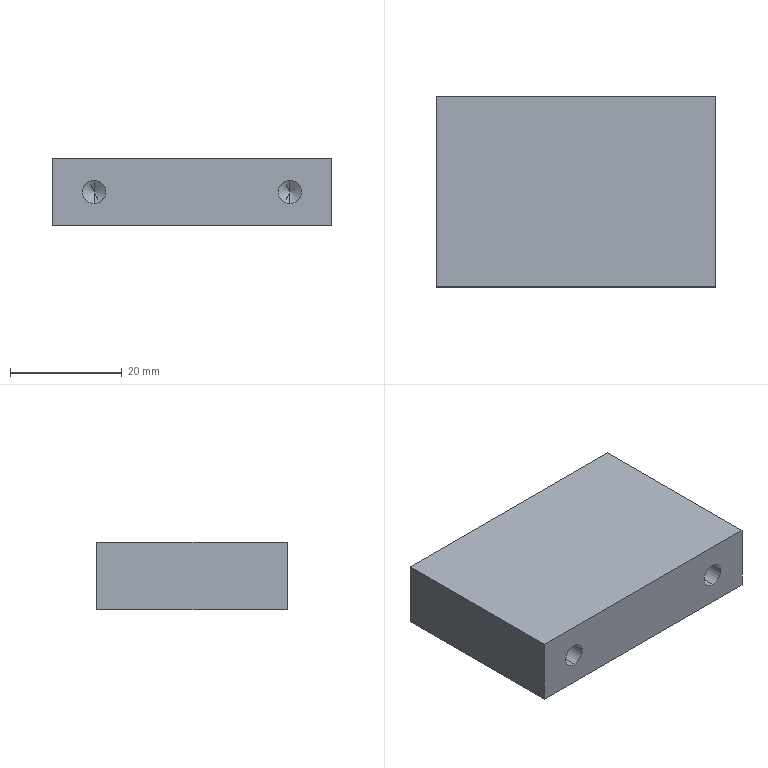Part | SolidWorks | features Extrusion 1, HoleWzd 1, MirrorPattern 1 | 1 solid | 22 faces | box 50 x 34 x 12 mm | volume 19690 mm3 | cylinder 8 | cone 8 | plane 6 | commonest cylinder face diameters 4.2 x8
STEP:
#1=CARTESIAN_POINT('',(-17.5,4.6,-2.1));
#2=VERTEX_POINT('',#1);
#3=CARTESIAN_POINT('',(-17.5,4.6,2.1));
#4=VERTEX_POINT('',#3);
#5=CARTESIAN_POINT('',(-17.5,4.6,0.));
#6=DIRECTION('',(0.,1.,0.));
#7=DIRECTION('',(0.,0.,1.));
#8=AXIS2_PLACEMENT_3D('',#5,#6,#7);
#9=CIRCLE('',#8,2.1);
#10=EDGE_CURVE('',#2,#4,#9,.T.);
#11=ORIENTED_EDGE('',*,*,#10,.F.);
#12=CARTESIAN_POINT('',(-17.5,17.,-2.1));
#13=VERTEX_POINT('',#12);
#14=CARTESIAN_POINT('',(-17.5,17.,-2.1));
#15=DIRECTION('',(0.,1.,0.));
#16=VECTOR('',#15,1000.);
#17=LINE('',#14,#16);
#18=EDGE_CURVE('',#2,#13,#17,.T.);
#19=ORIENTED_EDGE('',*,*,#18,.T.);
#20=CARTESIAN_POINT('',(-17.5,17.,2.1));
#21=VERTEX_POINT('',#20);
#22=CARTESIAN_POINT('',(-17.5,17.,0.));
#23=DIRECTION('',(0.,1.,0.));
#24=DIRECTION('',(0.,0.,1.));
#25=AXIS2_PLACEMENT_3D('',#22,#23,#24);
#26=CIRCLE('',#25,2.1);
#27=EDGE_CURVE('',#13,#21,#26,.T.);
#28=ORIENTED_EDGE('',*,*,#27,.T.);
#29=CARTESIAN_POINT('',(-17.5,17.,2.1));
#30=DIRECTION('',(0.,1.,0.));
#31=VECTOR('',#30,1000.);
#32=LINE('',#29,#31);
#33=EDGE_CURVE('',#4,#21,#32,.T.);
#34=ORIENTED_EDGE('',*,*,#33,.F.);
#35=EDGE_LOOP('',(#11,#19,#28,#34));
#36=FACE_OUTER_BOUND('',#35,.T.);
#37=CARTESIAN_POINT('',(-17.5,17.,0.));
#38=DIRECTION('',(0.,1.,0.));
#39=DIRECTION('',(0.,0.,1.));
#40=AXIS2_PLACEMENT_3D('',#37,#38,#39);
#41=CYLINDRICAL_SURFACE('',#40,2.1);
#42=ADVANCED_FACE('',(#36),#41,.F.);
#43=CARTESIAN_POINT('',(-17.5,3.338,0.));
#44=VERTEX_POINT('',#43);
#45=CARTESIAN_POINT('',(-17.5,4.6,2.1));
#46=DIRECTION('',(0.,0.515,0.8572));
#47=VECTOR('',#46,1000.);
#48=LINE('',#45,#47);
#49=EDGE_CURVE('',#44,#4,#48,.T.);
#50=ORIENTED_EDGE('',*,*,#49,.F.);
#51=CARTESIAN_POINT('',(-17.5,4.6,-2.1));
#52=DIRECTION('',(0.,0.515,-0.8572));
#53=VECTOR('',#52,1000.);
#54=LINE('',#51,#53);
#55=EDGE_CURVE('',#44,#2,#54,.T.);
#56=ORIENTED_EDGE('',*,*,#55,.T.);
#57=ORIENTED_EDGE('',*,*,#10,.T.);
#58=EDGE_LOOP('',(#50,#56,#57));
#59=FACE_OUTER_BOUND('',#58,.T.);
#60=CARTESIAN_POINT('',(-17.5,4.6,0.));
#61=DIRECTION('',(0.,1.,0.));
#62=DIRECTION('',(0.,0.,1.));
#63=AXIS2_PLACEMENT_3D('',#60,#61,#62);
#64=CONICAL_SURFACE('',#63,2.1,1.03);
#65=ADVANCED_FACE('',(#59),#64,.F.);
#66=CARTESIAN_POINT('',(17.5,4.6,-2.1));
#67=VERTEX_POINT('',#66);
#68=CARTESIAN_POINT('',(17.5,4.6,2.1));
#69=VERTEX_POINT('',#68);
#70=CARTESIAN_POINT('',(17.5,4.6,0.));
#71=DIRECTION('',(0.,1.,0.));
#72=DIRECTION('',(0.,0.,1.));
#73=AXIS2_PLACEMENT_3D('',#70,#71,#72);
#74=CIRCLE('',#73,2.1);
#75=EDGE_CURVE('',#67,#69,#74,.T.);
#76=ORIENTED_EDGE('',*,*,#75,.F.);
#77=CARTESIAN_POINT('',(17.5,17.,-2.1));
#78=VERTEX_POINT('',#77);
#79=CARTESIAN_POINT('',(17.5,17.,-2.1));
#80=DIRECTION('',(0.,1.,0.));
#81=VECTOR('',#80,1000.);
#82=LINE('',#79,#81);
#83=EDGE_CURVE('',#67,#78,#82,.T.);
#84=ORIENTED_EDGE('',*,*,#83,.T.);
#85=CARTESIAN_POINT('',(17.5,17.,2.1));
#86=VERTEX_POINT('',#85);
#87=CARTESIAN_POINT('',(17.5,17.,0.));
#88=DIRECTION('',(0.,1.,0.));
#89=DIRECTION('',(0.,0.,1.));
#90=AXIS2_PLACEMENT_3D('',#87,#88,#89);
#91=CIRCLE('',#90,2.1);
#92=EDGE_CURVE('',#78,#86,#91,.T.);
#93=ORIENTED_EDGE('',*,*,#92,.T.);
#94=CARTESIAN_POINT('',(17.5,17.,2.1));
#95=DIRECTION('',(0.,1.,0.));
#96=VECTOR('',#95,1000.);
#97=LINE('',#94,#96);
#98=EDGE_CURVE('',#69,#86,#97,.T.);
#99=ORIENTED_EDGE('',*,*,#98,.F.);
#100=EDGE_LOOP('',(#76,#84,#93,#99));
#101=FACE_OUTER_BOUND('',#100,.T.);
#102=CARTESIAN_POINT('',(17.5,17.,0.));
#103=DIRECTION('',(0.,1.,0.));
#104=DIRECTION('',(0.,0.,1.));
#105=AXIS2_PLACEMENT_3D('',#102,#103,#104);
#106=CYLINDRICAL_SURFACE('',#105,2.1);
#107=ADVANCED_FACE('',(#101),#106,.F.);
#108=CARTESIAN_POINT('',(17.5,3.338,0.));
#109=VERTEX_POINT('',#108);
#110=CARTESIAN_POINT('',(17.5,4.6,2.1));
#111=DIRECTION('',(0.,0.515,0.8572));
#112=VECTOR('',#111,1000.);
#113=LINE('',#110,#112);
#114=EDGE_CURVE('',#109,#69,#113,.T.);
#115=ORIENTED_EDGE('',*,*,#114,.F.);
#116=CARTESIAN_POINT('',(17.5,4.6,-2.1));
#117=DIRECTION('',(0.,0.515,-0.8572));
#118=VECTOR('',#117,1000.);
#119=LINE('',#116,#118);
#120=EDGE_CURVE('',#109,#67,#119,.T.);
#121=ORIENTED_EDGE('',*,*,#120,.T.);
#122=ORIENTED_EDGE('',*,*,#75,.T.);
#123=EDGE_LOOP('',(#115,#121,#122));
#124=FACE_OUTER_BOUND('',#123,.T.);
#125=CARTESIAN_POINT('',(17.5,4.6,0.));
#126=DIRECTION('',(0.,1.,0.));
#127=DIRECTION('',(0.,0.,1.));
#128=AXIS2_PLACEMENT_3D('',#125,#126,#127);
#129=CONICAL_SURFACE('',#128,2.1,1.03);
#130=ADVANCED_FACE('',(#124),#129,.F.);
#131=CARTESIAN_POINT('',(-17.5,-4.6,2.1));
#132=VERTEX_POINT('',#131);
#133=CARTESIAN_POINT('',(-17.5,-4.6,-2.1));
#134=VERTEX_POINT('',#133);
#135=CARTESIAN_POINT('',(-17.5,-4.6,0.));
#136=DIRECTION('',(0.,-1.,0.));
#137=DIRECTION('',(0.,0.,-1.));
#138=AXIS2_PLACEMENT_3D('',#135,#136,#137);
#139=CIRCLE('',#138,2.1);
#140=EDGE_CURVE('',#132,#134,#139,.T.);
#141=ORIENTED_EDGE('',*,*,#140,.F.);
#142=CARTESIAN_POINT('',(-17.5,-17.,2.1));
#143=VERTEX_POINT('',#142);
#144=CARTESIAN_POINT('',(-17.5,-17.,2.1));
#145=DIRECTION('',(0.,-1.,0.));
#146=VECTOR('',#145,1000.);
#147=LINE('',#144,#146);
#148=EDGE_CURVE('',#132,#143,#147,.T.);
#149=ORIENTED_EDGE('',*,*,#148,.T.);
#150=CARTESIAN_POINT('',(-17.5,-17.,-2.1));
#151=VERTEX_POINT('',#150);
#152=CARTESIAN_POINT('',(-17.5,-17.,0.));
#153=DIRECTION('',(0.,-1.,0.));
#154=DIRECTION('',(0.,0.,-1.));
#155=AXIS2_PLACEMENT_3D('',#152,#153,#154);
#156=CIRCLE('',#155,2.1);
#157=EDGE_CURVE('',#143,#151,#156,.T.);
#158=ORIENTED_EDGE('',*,*,#157,.T.);
#159=CARTESIAN_POINT('',(-17.5,-17.,-2.1));
#160=DIRECTION('',(0.,-1.,0.));
#161=VECTOR('',#160,1000.);
#162=LINE('',#159,#161);
#163=EDGE_CURVE('',#134,#151,#162,.T.);
#164=ORIENTED_EDGE('',*,*,#163,.F.);
#165=EDGE_LOOP('',(#141,#149,#158,#164));
#166=FACE_OUTER_BOUND('',#165,.T.);
#167=CARTESIAN_POINT('',(-17.5,-17.,0.));
#168=DIRECTION('',(0.,-1.,0.));
#169=DIRECTION('',(0.,0.,-1.));
#170=AXIS2_PLACEMENT_3D('',#167,#168,#169);
#171=CYLINDRICAL_SURFACE('',#170,2.1);
#172=ADVANCED_FACE('',(#166),#171,.F.);
#173=CARTESIAN_POINT('',(-17.5,-3.338,0.));
#174=VERTEX_POINT('',#173);
#175=CARTESIAN_POINT('',(-17.5,-4.6,-2.1));
#176=DIRECTION('',(0.,-0.515,-0.8572));
#177=VECTOR('',#176,1000.);
#178=LINE('',#175,#177);
#179=EDGE_CURVE('',#174,#134,#178,.T.);
#180=ORIENTED_EDGE('',*,*,#179,.F.);
#181=CARTESIAN_POINT('',(-17.5,-4.6,2.1));
#182=DIRECTION('',(0.,-0.515,0.8572));
#183=VECTOR('',#182,1000.);
#184=LINE('',#181,#183);
#185=EDGE_CURVE('',#174,#132,#184,.T.);
#186=ORIENTED_EDGE('',*,*,#185,.T.);
#187=ORIENTED_EDGE('',*,*,#140,.T.);
#188=EDGE_LOOP('',(#180,#186,#187));
#189=FACE_OUTER_BOUND('',#188,.T.);
#190=CARTESIAN_POINT('',(-17.5,-4.6,0.));
#191=DIRECTION('',(0.,-1.,0.));
#192=DIRECTION('',(0.,0.,-1.));
#193=AXIS2_PLACEMENT_3D('',#190,#191,#192);
#194=CONICAL_SURFACE('',#193,2.1,1.03);
#195=ADVANCED_FACE('',(#189),#194,.F.);
#196=CARTESIAN_POINT('',(17.5,-4.6,2.1));
#197=VERTEX_POINT('',#196);
#198=CARTESIAN_POINT('',(17.5,-4.6,-2.1));
#199=VERTEX_POINT('',#198);
#200=CARTESIAN_POINT('',(17.5,-4.6,0.));
#201=DIRECTION('',(0.,-1.,0.));
#202=DIRECTION('',(0.,0.,-1.));
#203=AXIS2_PLACEMENT_3D('',#200,#201,#202);
#204=CIRCLE('',#203,2.1);
#205=EDGE_CURVE('',#197,#199,#204,.T.);
#206=ORIENTED_EDGE('',*,*,#205,.F.);
#207=CARTESIAN_POINT('',(17.5,-17.,2.1));
#208=VERTEX_POINT('',#207);
#209=CARTESIAN_POINT('',(17.5,-17.,2.1));
#210=DIRECTION('',(0.,-1.,0.));
#211=VECTOR('',#210,1000.);
#212=LINE('',#209,#211);
#213=EDGE_CURVE('',#197,#208,#212,.T.);
#214=ORIENTED_EDGE('',*,*,#213,.T.);
#215=CARTESIAN_POINT('',(17.5,-17.,-2.1));
#216=VERTEX_POINT('',#215);
#217=CARTESIAN_POINT('',(17.5,-17.,0.));
#218=DIRECTION('',(0.,-1.,0.));
#219=DIRECTION('',(0.,0.,-1.));
#220=AXIS2_PLACEMENT_3D('',#217,#218,#219);
#221=CIRCLE('',#220,2.1);
#222=EDGE_CURVE('',#208,#216,#221,.T.);
#223=ORIENTED_EDGE('',*,*,#222,.T.);
#224=CARTESIAN_POINT('',(17.5,-17.,-2.1));
#225=DIRECTION('',(0.,-1.,0.));
#226=VECTOR('',#225,1000.);
#227=LINE('',#224,#226);
#228=EDGE_CURVE('',#199,#216,#227,.T.);
#229=ORIENTED_EDGE('',*,*,#228,.F.);
#230=EDGE_LOOP('',(#206,#214,#223,#229));
#231=FACE_OUTER_BOUND('',#230,.T.);
#232=CARTESIAN_POINT('',(17.5,-17.,0.));
#233=DIRECTION('',(0.,-1.,0.));
#234=DIRECTION('',(0.,0.,-1.));
#235=AXIS2_PLACEMENT_3D('',#232,#233,#234);
#236=CYLINDRICAL_SURFACE('',#235,2.1);
#237=ADVANCED_FACE('',(#231),#236,.F.);
#238=CARTESIAN_POINT('',(17.5,-3.338,0.));
#239=VERTEX_POINT('',#238);
#240=CARTESIAN_POINT('',(17.5,-4.6,-2.1));
#241=DIRECTION('',(0.,-0.515,-0.8572));
#242=VECTOR('',#241,1000.);
#243=LINE('',#240,#242);
#244=EDGE_CURVE('',#239,#199,#243,.T.);
#245=ORIENTED_EDGE('',*,*,#244,.F.);
#246=CARTESIAN_POINT('',(17.5,-4.6,2.1));
#247=DIRECTION('',(0.,-0.515,0.8572));
#248=VECTOR('',#247,1000.);
#249=LINE('',#246,#248);
#250=EDGE_CURVE('',#239,#197,#249,.T.);
#251=ORIENTED_EDGE('',*,*,#250,.T.);
#252=ORIENTED_EDGE('',*,*,#205,.T.);
#253=EDGE_LOOP('',(#245,#251,#252));
#254=FACE_OUTER_BOUND('',#253,.T.);
#255=CARTESIAN_POINT('',(17.5,-4.6,0.));
#256=DIRECTION('',(0.,-1.,0.));
#257=DIRECTION('',(0.,0.,-1.));
#258=AXIS2_PLACEMENT_3D('',#255,#256,#257);
#259=CONICAL_SURFACE('',#258,2.1,1.03);
#260=ADVANCED_FACE('',(#254),#259,.F.);
#261=CARTESIAN_POINT('',(25.,-17.,-6.));
#262=VERTEX_POINT('',#261);
#263=CARTESIAN_POINT('',(25.,17.,-6.));
#264=VERTEX_POINT('',#263);
#265=CARTESIAN_POINT('',(25.,-17.,-6.));
#266=DIRECTION('',(0.,1.,0.));
#267=VECTOR('',#266,1000.);
#268=LINE('',#265,#267);
#269=EDGE_CURVE('',#262,#264,#268,.T.);
#270=ORIENTED_EDGE('',*,*,#269,.T.);
#271=CARTESIAN_POINT('',(25.,17.,6.));
#272=VERTEX_POINT('',#271);
#273=CARTESIAN_POINT('',(25.,17.,6.));
#274=DIRECTION('',(0.,0.,-1.));
#275=VECTOR('',#274,1000.);
#276=LINE('',#273,#275);
#277=EDGE_CURVE('',#272,#264,#276,.T.);
#278=ORIENTED_EDGE('',*,*,#277,.F.);
#279=CARTESIAN_POINT('',(25.,-17.,6.));
#280=VERTEX_POINT('',#279);
#281=CARTESIAN_POINT('',(25.,-17.,6.));
#282=DIRECTION('',(0.,1.,0.));
#283=VECTOR('',#282,1000.);
#284=LINE('',#281,#283);
#285=EDGE_CURVE('',#280,#272,#284,.T.);
#286=ORIENTED_EDGE('',*,*,#285,.F.);
#287=CARTESIAN_POINT('',(25.,-17.,6.));
#288=DIRECTION('',(0.,0.,-1.));
#289=VECTOR('',#288,1000.);
#290=LINE('',#287,#289);
#291=EDGE_CURVE('',#280,#262,#290,.T.);
#292=ORIENTED_EDGE('',*,*,#291,.T.);
#293=EDGE_LOOP('',(#270,#278,#286,#292));
#294=FACE_OUTER_BOUND('',#293,.T.);
#295=CARTESIAN_POINT('',(25.,-17.,6.));
#296=DIRECTION('',(-1.,0.,0.));
#297=DIRECTION('',(0.,0.,1.));
#298=AXIS2_PLACEMENT_3D('',#295,#296,#297);
#299=PLANE('',#298);
#300=ADVANCED_FACE('',(#294),#299,.F.);
#301=CARTESIAN_POINT('',(-17.5,17.,0.));
#302=DIRECTION('',(0.,1.,0.));
#303=DIRECTION('',(0.,0.,1.));
#304=AXIS2_PLACEMENT_3D('',#301,#302,#303);
#305=CIRCLE('',#304,2.1);
#306=EDGE_CURVE('',#21,#13,#305,.T.);
#307=ORIENTED_EDGE('',*,*,#306,.F.);
#308=ORIENTED_EDGE('',*,*,#27,.F.);
#309=EDGE_LOOP('',(#307,#308));
#310=FACE_BOUND('',#309,.T.);
#311=CARTESIAN_POINT('',(17.5,17.,0.));
#312=DIRECTION('',(0.,1.,0.));
#313=DIRECTION('',(0.,0.,1.));
#314=AXIS2_PLACEMENT_3D('',#311,#312,#313);
#315=CIRCLE('',#314,2.1);
#316=EDGE_CURVE('',#86,#78,#315,.T.);
#317=ORIENTED_EDGE('',*,*,#316,.F.);
#318=ORIENTED_EDGE('',*,*,#92,.F.);
#319=EDGE_LOOP('',(#317,#318));
#320=FACE_BOUND('',#319,.T.);
#321=CARTESIAN_POINT('',(-25.,17.,-6.));
#322=VERTEX_POINT('',#321);
#323=CARTESIAN_POINT('',(-25.,17.,-6.));
#324=DIRECTION('',(-1.,0.,0.));
#325=VECTOR('',#324,1000.);
#326=LINE('',#323,#325);
#327=EDGE_CURVE('',#264,#322,#326,.T.);
#328=ORIENTED_EDGE('',*,*,#327,.T.);
#329=CARTESIAN_POINT('',(-25.,17.,6.));
#330=VERTEX_POINT('',#329);
#331=CARTESIAN_POINT('',(-25.,17.,6.));
#332=DIRECTION('',(0.,0.,-1.));
#333=VECTOR('',#332,1000.);
#334=LINE('',#331,#333);
#335=EDGE_CURVE('',#330,#322,#334,.T.);
#336=ORIENTED_EDGE('',*,*,#335,.F.);
#337=CARTESIAN_POINT('',(-25.,17.,6.));
#338=DIRECTION('',(-1.,0.,0.));
#339=VECTOR('',#338,1000.);
#340=LINE('',#337,#339);
#341=EDGE_CURVE('',#272,#330,#340,.T.);
#342=ORIENTED_EDGE('',*,*,#341,.F.);
#343=ORIENTED_EDGE('',*,*,#277,.T.);
#344=EDGE_LOOP('',(#328,#336,#342,#343));
#345=FACE_OUTER_BOUND('',#344,.T.);
#346=CARTESIAN_POINT('',(-25.,17.,6.));
#347=DIRECTION('',(0.,-1.,0.));
#348=DIRECTION('',(0.,0.,-1.));
#349=AXIS2_PLACEMENT_3D('',#346,#347,#348);
#350=PLANE('',#349);
#351=ADVANCED_FACE('',(#310,#320,#345),#350,.F.);
#352=CARTESIAN_POINT('',(-25.,-17.,-6.));
#353=VERTEX_POINT('',#352);
#354=CARTESIAN_POINT('',(-25.,-17.,-6.));
#355=DIRECTION('',(0.,-1.,0.));
#356=VECTOR('',#355,1000.);
#357=LINE('',#354,#356);
#358=EDGE_CURVE('',#322,#353,#357,.T.);
#359=ORIENTED_EDGE('',*,*,#358,.T.);
#360=CARTESIAN_POINT('',(-25.,-17.,6.));
#361=VERTEX_POINT('',#360);
#362=CARTESIAN_POINT('',(-25.,-17.,6.));
#363=DIRECTION('',(0.,0.,-1.));
#364=VECTOR('',#363,1000.);
#365=LINE('',#362,#364);
#366=EDGE_CURVE('',#361,#353,#365,.T.);
#367=ORIENTED_EDGE('',*,*,#366,.F.);
#368=CARTESIAN_POINT('',(-25.,-17.,6.));
#369=DIRECTION('',(0.,-1.,0.));
#370=VECTOR('',#369,1000.);
#371=LINE('',#368,#370);
#372=EDGE_CURVE('',#330,#361,#371,.T.);
#373=ORIENTED_EDGE('',*,*,#372,.F.);
#374=ORIENTED_EDGE('',*,*,#335,.T.);
#375=EDGE_LOOP('',(#359,#367,#373,#374));
#376=FACE_OUTER_BOUND('',#375,.T.);
#377=CARTESIAN_POINT('',(-25.,-17.,6.));
#378=DIRECTION('',(1.,0.,0.));
#379=DIRECTION('',(0.,0.,-1.));
#380=AXIS2_PLACEMENT_3D('',#377,#378,#379);
#381=PLANE('',#380);
#382=ADVANCED_FACE('',(#376),#381,.F.);
#383=CARTESIAN_POINT('',(-17.5,-17.,0.));
#384=DIRECTION('',(0.,-1.,0.));
#385=DIRECTION('',(0.,0.,-1.));
#386=AXIS2_PLACEMENT_3D('',#383,#384,#385);
#387=CIRCLE('',#386,2.1);
#388=EDGE_CURVE('',#151,#143,#387,.T.);
#389=ORIENTED_EDGE('',*,*,#388,.F.);
#390=ORIENTED_EDGE('',*,*,#157,.F.);
#391=EDGE_LOOP('',(#389,#390));
#392=FACE_BOUND('',#391,.T.);
#393=CARTESIAN_POINT('',(17.5,-17.,0.));
#394=DIRECTION('',(0.,-1.,0.));
#395=DIRECTION('',(0.,0.,-1.));
#396=AXIS2_PLACEMENT_3D('',#393,#394,#395);
#397=CIRCLE('',#396,2.1);
#398=EDGE_CURVE('',#216,#208,#397,.T.);
#399=ORIENTED_EDGE('',*,*,#398,.F.);
#400=ORIENTED_EDGE('',*,*,#222,.F.);
#401=EDGE_LOOP('',(#399,#400));
#402=FACE_BOUND('',#401,.T.);
#403=CARTESIAN_POINT('',(-25.,-17.,-6.));
#404=DIRECTION('',(1.,0.,0.));
#405=VECTOR('',#404,1000.);
#406=LINE('',#403,#405);
#407=EDGE_CURVE('',#353,#262,#406,.T.);
#408=ORIENTED_EDGE('',*,*,#407,.T.);
#409=ORIENTED_EDGE('',*,*,#291,.F.);
#410=CARTESIAN_POINT('',(-25.,-17.,6.));
#411=DIRECTION('',(1.,0.,0.));
#412=VECTOR('',#411,1000.);
#413=LINE('',#410,#412);
#414=EDGE_CURVE('',#361,#280,#413,.T.);
#415=ORIENTED_EDGE('',*,*,#414,.F.);
#416=ORIENTED_EDGE('',*,*,#366,.T.);
#417=EDGE_LOOP('',(#408,#409,#415,#416));
#418=FACE_OUTER_BOUND('',#417,.T.);
#419=CARTESIAN_POINT('',(-25.,-17.,6.));
#420=DIRECTION('',(0.,1.,0.));
#421=DIRECTION('',(0.,0.,1.));
#422=AXIS2_PLACEMENT_3D('',#419,#420,#421);
#423=PLANE('',#422);
#424=ADVANCED_FACE('',(#392,#402,#418),#423,.F.);
#425=ORIENTED_EDGE('',*,*,#285,.T.);
#426=ORIENTED_EDGE('',*,*,#341,.T.);
#427=ORIENTED_EDGE('',*,*,#372,.T.);
#428=ORIENTED_EDGE('',*,*,#414,.T.);
#429=EDGE_LOOP('',(#425,#426,#427,#428));
#430=FACE_OUTER_BOUND('',#429,.T.);
#431=CARTESIAN_POINT('',(0.,0.,6.));
#432=DIRECTION('',(0.,0.,-1.));
#433=DIRECTION('',(-1.,0.,0.));
#434=AXIS2_PLACEMENT_3D('',#431,#432,#433);
#435=PLANE('',#434);
#436=ADVANCED_FACE('',(#430),#435,.F.);
#437=ORIENTED_EDGE('',*,*,#269,.F.);
#438=ORIENTED_EDGE('',*,*,#407,.F.);
#439=ORIENTED_EDGE('',*,*,#358,.F.);
#440=ORIENTED_EDGE('',*,*,#327,.F.);
#441=EDGE_LOOP('',(#437,#438,#439,#440));
#442=FACE_OUTER_BOUND('',#441,.T.);
#443=CARTESIAN_POINT('',(0.,0.,-6.));
#444=DIRECTION('',(0.,0.,-1.));
#445=DIRECTION('',(-1.,0.,0.));
#446=AXIS2_PLACEMENT_3D('',#443,#444,#445);
#447=PLANE('',#446);
#448=ADVANCED_FACE('',(#442),#447,.T.);
#449=ORIENTED_EDGE('',*,*,#250,.F.);
#450=ORIENTED_EDGE('',*,*,#244,.T.);
#451=CARTESIAN_POINT('',(17.5,-4.6,0.));
#452=DIRECTION('',(0.,-1.,0.));
#453=DIRECTION('',(0.,0.,-1.));
#454=AXIS2_PLACEMENT_3D('',#451,#452,#453);
#455=CIRCLE('',#454,2.1);
#456=EDGE_CURVE('',#199,#197,#455,.T.);
#457=ORIENTED_EDGE('',*,*,#456,.T.);
#458=EDGE_LOOP('',(#449,#450,#457));
#459=FACE_OUTER_BOUND('',#458,.T.);
#460=CARTESIAN_POINT('',(17.5,-4.6,0.));
#461=DIRECTION('',(0.,-1.,0.));
#462=DIRECTION('',(0.,0.,-1.));
#463=AXIS2_PLACEMENT_3D('',#460,#461,#462);
#464=CONICAL_SURFACE('',#463,2.1,1.03);
#465=ADVANCED_FACE('',(#459),#464,.F.);
#466=ORIENTED_EDGE('',*,*,#213,.F.);
#467=ORIENTED_EDGE('',*,*,#456,.F.);
#468=ORIENTED_EDGE('',*,*,#228,.T.);
#469=ORIENTED_EDGE('',*,*,#398,.T.);
#470=EDGE_LOOP('',(#466,#467,#468,#469));
#471=FACE_OUTER_BOUND('',#470,.T.);
#472=CARTESIAN_POINT('',(17.5,-17.,0.));
#473=DIRECTION('',(0.,-1.,0.));
#474=DIRECTION('',(0.,0.,-1.));
#475=AXIS2_PLACEMENT_3D('',#472,#473,#474);
#476=CYLINDRICAL_SURFACE('',#475,2.1);
#477=ADVANCED_FACE('',(#471),#476,.F.);
#478=ORIENTED_EDGE('',*,*,#185,.F.);
#479=ORIENTED_EDGE('',*,*,#179,.T.);
#480=CARTESIAN_POINT('',(-17.5,-4.6,0.));
#481=DIRECTION('',(0.,-1.,0.));
#482=DIRECTION('',(0.,0.,-1.));
#483=AXIS2_PLACEMENT_3D('',#480,#481,#482);
#484=CIRCLE('',#483,2.1);
#485=EDGE_CURVE('',#134,#132,#484,.T.);
#486=ORIENTED_EDGE('',*,*,#485,.T.);
#487=EDGE_LOOP('',(#478,#479,#486));
#488=FACE_OUTER_BOUND('',#487,.T.);
#489=CARTESIAN_POINT('',(-17.5,-4.6,0.));
#490=DIRECTION('',(0.,-1.,0.));
#491=DIRECTION('',(0.,0.,-1.));
#492=AXIS2_PLACEMENT_3D('',#489,#490,#491);
#493=CONICAL_SURFACE('',#492,2.1,1.03);
#494=ADVANCED_FACE('',(#488),#493,.F.);
#495=ORIENTED_EDGE('',*,*,#148,.F.);
#496=ORIENTED_EDGE('',*,*,#485,.F.);
#497=ORIENTED_EDGE('',*,*,#163,.T.);
#498=ORIENTED_EDGE('',*,*,#388,.T.);
#499=EDGE_LOOP('',(#495,#496,#497,#498));
#500=FACE_OUTER_BOUND('',#499,.T.);
#501=CARTESIAN_POINT('',(-17.5,-17.,0.));
#502=DIRECTION('',(0.,-1.,0.));
#503=DIRECTION('',(0.,0.,-1.));
#504=AXIS2_PLACEMENT_3D('',#501,#502,#503);
#505=CYLINDRICAL_SURFACE('',#504,2.1);
#506=ADVANCED_FACE('',(#500),#505,.F.);
#507=ORIENTED_EDGE('',*,*,#120,.F.);
#508=ORIENTED_EDGE('',*,*,#114,.T.);
#509=CARTESIAN_POINT('',(17.5,4.6,0.));
#510=DIRECTION('',(0.,1.,0.));
#511=DIRECTION('',(0.,0.,1.));
#512=AXIS2_PLACEMENT_3D('',#509,#510,#511);
#513=CIRCLE('',#512,2.1);
#514=EDGE_CURVE('',#69,#67,#513,.T.);
#515=ORIENTED_EDGE('',*,*,#514,.T.);
#516=EDGE_LOOP('',(#507,#508,#515));
#517=FACE_OUTER_BOUND('',#516,.T.);
#518=CARTESIAN_POINT('',(17.5,4.6,0.));
#519=DIRECTION('',(0.,1.,0.));
#520=DIRECTION('',(0.,0.,1.));
#521=AXIS2_PLACEMENT_3D('',#518,#519,#520);
#522=CONICAL_SURFACE('',#521,2.1,1.03);
#523=ADVANCED_FACE('',(#517),#522,.F.);
#524=ORIENTED_EDGE('',*,*,#83,.F.);
#525=ORIENTED_EDGE('',*,*,#514,.F.);
#526=ORIENTED_EDGE('',*,*,#98,.T.);
#527=ORIENTED_EDGE('',*,*,#316,.T.);
#528=EDGE_LOOP('',(#524,#525,#526,#527));
#529=FACE_OUTER_BOUND('',#528,.T.);
#530=CARTESIAN_POINT('',(17.5,17.,0.));
#531=DIRECTION('',(0.,1.,0.));
#532=DIRECTION('',(0.,0.,1.));
#533=AXIS2_PLACEMENT_3D('',#530,#531,#532);
#534=CYLINDRICAL_SURFACE('',#533,2.1);
#535=ADVANCED_FACE('',(#529),#534,.F.);
#536=ORIENTED_EDGE('',*,*,#55,.F.);
#537=ORIENTED_EDGE('',*,*,#49,.T.);
#538=CARTESIAN_POINT('',(-17.5,4.6,0.));
#539=DIRECTION('',(0.,1.,0.));
#540=DIRECTION('',(0.,0.,1.));
#541=AXIS2_PLACEMENT_3D('',#538,#539,#540);
#542=CIRCLE('',#541,2.1);
#543=EDGE_CURVE('',#4,#2,#542,.T.);
#544=ORIENTED_EDGE('',*,*,#543,.T.);
#545=EDGE_LOOP('',(#536,#537,#544));
#546=FACE_OUTER_BOUND('',#545,.T.);
#547=CARTESIAN_POINT('',(-17.5,4.6,0.));
#548=DIRECTION('',(0.,1.,0.));
#549=DIRECTION('',(0.,0.,1.));
#550=AXIS2_PLACEMENT_3D('',#547,#548,#549);
#551=CONICAL_SURFACE('',#550,2.1,1.03);
#552=ADVANCED_FACE('',(#546),#551,.F.);
#553=ORIENTED_EDGE('',*,*,#18,.F.);
#554=ORIENTED_EDGE('',*,*,#543,.F.);
#555=ORIENTED_EDGE('',*,*,#33,.T.);
#556=ORIENTED_EDGE('',*,*,#306,.T.);
#557=EDGE_LOOP('',(#553,#554,#555,#556));
#558=FACE_OUTER_BOUND('',#557,.T.);
#559=CARTESIAN_POINT('',(-17.5,17.,0.));
#560=DIRECTION('',(0.,1.,0.));
#561=DIRECTION('',(0.,0.,1.));
#562=AXIS2_PLACEMENT_3D('',#559,#560,#561);
#563=CYLINDRICAL_SURFACE('',#562,2.1);
#564=ADVANCED_FACE('',(#558),#563,.F.);
#565=CLOSED_SHELL('',(#42,#65,#107,#130,#172,#195,#237,#260,#300,#351,#382,#424,#436,#448,#465,#477,#494,#506,#523,#535,#552,#564));
#566=MANIFOLD_SOLID_BREP('',#565);
#567=CARTESIAN_POINT('',(0.,0.,0.));
#568=DIRECTION('',(0.,0.,1.));
#569=DIRECTION('',(1.,0.,0.));
#570=AXIS2_PLACEMENT_3D('',#567,#568,#569);
#571=(LENGTH_UNIT()NAMED_UNIT(*)SI_UNIT(.MILLI.,.METRE.));
#572=UNCERTAINTY_MEASURE_WITH_UNIT(LENGTH_MEASURE(0.00001),#571,'','');
#573=(NAMED_UNIT(*)PLANE_ANGLE_UNIT()SI_UNIT($,.RADIAN.));
#574=(NAMED_UNIT(*)SI_UNIT($,.STERADIAN.)SOLID_ANGLE_UNIT());
#575=(GEOMETRIC_REPRESENTATION_CONTEXT(3)GLOBAL_UNCERTAINTY_ASSIGNED_CONTEXT((#572))GLOBAL_UNIT_ASSIGNED_CONTEXT((#571,#573,#574))REPRESENTATION_CONTEXT('',''));
#576=ADVANCED_BREP_SHAPE_REPRESENTATION('',(#566,#570),#575);